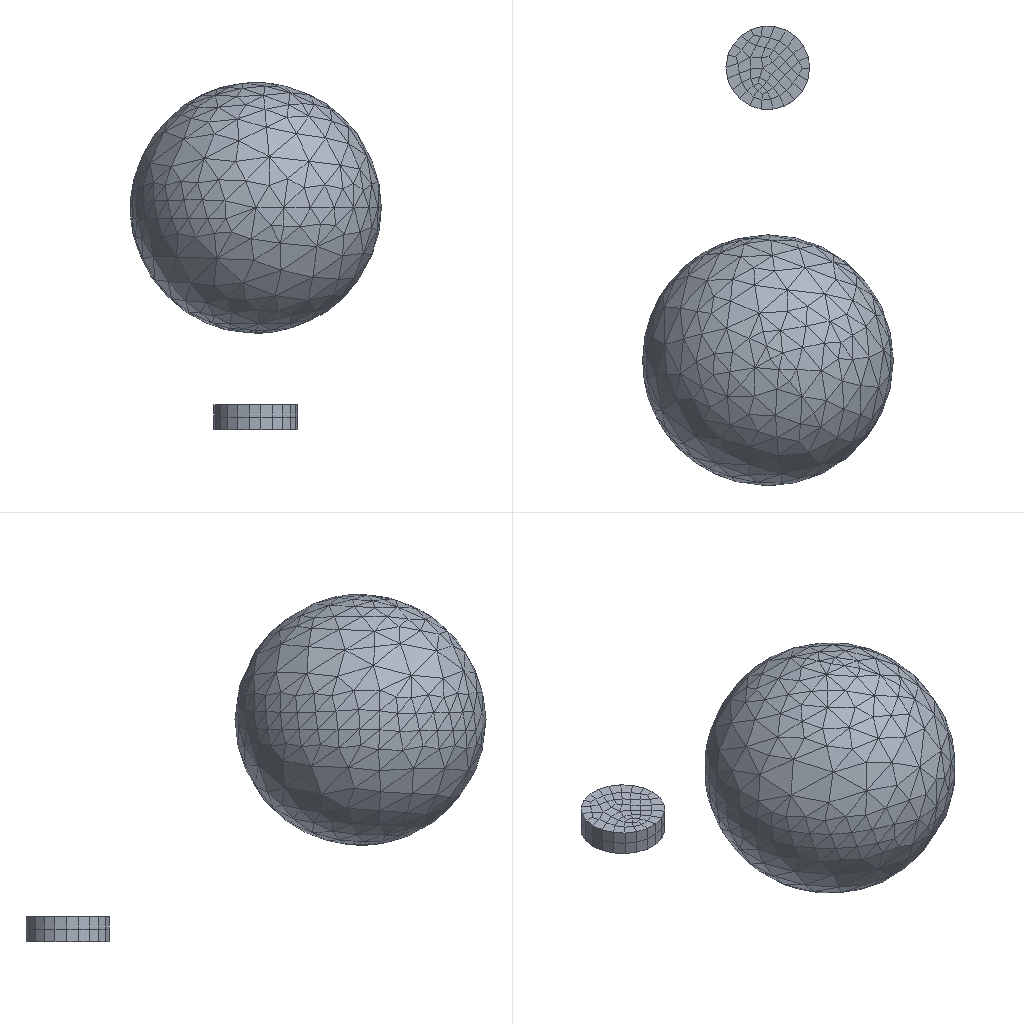Simulation study | abaqus
Set-up summary:
category,name,step,type,value,unit,region
solver,abaqus
solver,version,,,Abaqus/Explicit 2020
units,not stated in the deck,,not stated
analysis,deck,,transient,transient
load_step,Step-1,Step-1,transient
load_step,requested,,,1
mesh,nodes,,,6310
mesh,elements,,,4417
element_type,R3D4,,rigid,116
element_type,T3D2,,truss,568
element_type,C3D8R,,solid,116
element_type,C3D10M,,solid,3617
load,load commands in deck,,count,2
bc,support commands in deck,,count,7
material,RUBBER,,in results
material,STRING,,in results
check,setup vs results,,match,"per instance, exact: element labels, types and connectivity; labels of the nodes the elements use; coordinates of those nodes at SINGLE_PRECISION in 3 of 5 instance(s)"
Abaqus input file, long lists of numbers shortened:
*Heading
** Job name: Job-2 Model name: tennis_gcont
** Generated by: Abaqus/CAE 2020
*Preprint, echo=NO, model=NO, history=NO, contact=NO
**
** PARTS
**
*Part, name=FRAME
*Node
    105,  -2.16,  -7.3,           0.
    106,        -1.62,  -7.825,           0.
** (173 more lines like these left out)
*Element, type=R3D4
3001,   105,   106, 10106, 10105
3002,   106,   107, 10107, 10106
** (114 more lines like these left out)
*Nset, nset=FRAME-RefPt_, internal
 10000,
*End Part
**
*Part, name=PART-1
*Node
    104,  -2.7,       -6.625,           0.
    105,  -2.16,  -7.3,           0.
** (329 more lines like these left out)
*Element, type=T3D2
   1,  204,  205
   2,  205,  206
** (566 more lines like these left out)
*Elset, elset=STRINGS
    1,    2,    3,    4,    5,    6,    7,    8,    9,   10,   11,   12,   13,   14,   15,   16
   17,   18,   19,   20,   21,   22,   23,   24,   25,   26,   27,   28,   29,   30,   31,   32
** (34 more lines like these left out)
*Elset, elset=Set-6
    1,    2,    3,    4,    5,    6,    7,    8,    9,   10,   11,   12,   13,   14,   15,   16
   17,   18,   19,   20,   21,   22,   23,   24,   25,   26,   27,   28,   29,   30,   31,   32
** (34 more lines like these left out)
*Elset, elset=Set-7
    1,    2,    3,    4,    5,    6,    7,    8,    9,   10,   11,   12,   13,   14,   15,   16
   17,   18,   19,   20,   21,   22,   23,   24,   25,   26,   27,   28,   29,   30,   31,   32
** (34 more lines like these left out)
** Section: Section-1-STRINGS
*Solid Section, elset=Set-7, material=STRING
0.007854,
*End Part
**
*Part, name=bizhen
*Node
      1,  0.4153, -0.2784,           0.
      2,  0.4769, -0.1501,           0.
** (138 more lines like these left out)
*Element, type=C3D8R
 1,  93,  90,  89,  94,  23,  20,  19,  24
 2,  94,  89,  88,  95,  24,  19,  18,  25
** (56 more lines like these left out)
*Nset, nset=Set-2, generate
   1,  140,    1
*Elset, elset=Set-2, generate
  1,  58,   1
** Section: Section-bizhen
*Solid Section, elset=Set-2, material=RUBBER
,
*End Part
**
*Part, name=qiu
*Node
      1,  0.3338,   1.462,           0.
      2,   0.6508,    1.351,           0.
** (5522 more lines like these left out)
*Element, type=C3D10M
   1,  337,  338,  339,  340,  790,  789,  788,  792,  791,  793
   2,  337,  341,  342,  343,  796,  795,  794,  798,  797,  799
** (3615 more lines like these left out)
*Nset, nset=Set-7, generate
    1,  5524,     1
*Elset, elset=Set-7, generate
    1,  3617,     1
*Nset, nset=Set-8, generate
    1,  5524,     1
*Elset, elset=Set-8, generate
    1,  3617,     1
** Section: Section-bizhen
*Solid Section, elset=Set-8, material=RUBBER
,
*End Part
**
**
** ASSEMBLY
**
*Assembly, name=Assembly
**
*Instance, name=FRAME-1, part=FRAME
*End Instance
**
*Instance, name=PART-1-1, part=PART-1
*End Instance
**
*Instance, name=bizhen-1, part=bizhen
          0.,          3.5,           0.
*End Instance
**
*Instance, name=bizhen-1-lin-2-1, part=bizhen
          0.,          3.5,        -0.15
*End Instance
**
*Instance, name=qiu-1, part=qiu
          0.,           0.,          2.5
*End Instance
**
*Node
      1,          1.5,           0.,          2.5
*Node
      2,           0.,           0.,           0.
*Nset, nset=BACK, instance=FRAME-1
 20105, 20106, 20107, 20108, 20109, 20110, 20111, 20112, 20113, 20204, 20214, 20303, 20315, 20402, 20416, 20501
 20517, 20601, 20617, 20701, 20717, 20801, 20817, 20901, 20917, 21001, 21017, 21101, 21117, 21201, 21217, 21301
** (2 more lines like these left out)
*Elset, elset=FRAME, instance=FRAME-1
 3001, 3002, 3003, 3004, 3005, 3006, 3007, 3008, 3009, 3010, 3011, 3012, 3013, 3014, 3015, 3016
 3017, 3018, 3019, 3020, 3021, 3022, 3023, 3024, 3025, 3036, 3037, 3038, 3039, 3040, 3041, 3042
** (6 more lines like these left out)
*Nset, nset=FRONT, instance=FRAME-1
 10105, 10106, 10107, 10108, 10109, 10110, 10111, 10112, 10113, 10204, 10214, 10303, 10315, 10402, 10416, 10501
 10517, 10601, 10617, 10701, 10717, 10801, 10817, 10901, 10917, 11001, 11017, 11101, 11117, 11201, 11217, 11301
** (2 more lines like these left out)
*Nset, nset=MIDPLANE, instance=FRAME-1
  105,  106,  107,  108,  109,  110,  111,  112,  113,  204,  214,  303,  315,  402,  416,  501
  517,  601,  617,  701,  717,  801,  817,  901,  917, 1001, 1017, 1101, 1117, 1201, 1217, 1301
** (2 more lines like these left out)
*Nset, nset=MIDPLANE, instance=PART-1-1
  105,  106,  107,  108,  109,  110,  111,  112,  113,  204,  214,  303,  315,  402,  416,  501
  517,  601,  617,  701,  717,  801,  817,  901,  917, 1001, 1017, 1101, 1117, 1201, 1217, 1301
** (2 more lines like these left out)
*Nset, nset=N200, instance=PART-1-1, generate
 204,  214,    1
*Nset, nset=N200, instance=FRAME-1
 204, 214
*Nset, nset=N500, instance=PART-1-1, generate
 502,  516,    1
*Nset, nset=N1900, instance=FRAME-1
 1902, 1916
*Nset, nset=N1900, instance=PART-1-1, generate
 1902,  1916,     1
*Nset, nset=NCONTACT, instance=PART-1-1
  205,  206,  207,  208,  209,  210,  211,  212,  213,  304,  305,  306,  307,  308,  309,  310
  311,  312,  313,  314,  403,  404,  405,  406,  407,  408,  409,  410,  411,  412,  413,  414
** (15 more lines like these left out)
*Nset, nset=STRINGS, instance=PART-1-1
  205,  206,  207,  208,  209,  210,  211,  212,  213,  304,  305,  306,  307,  308,  309,  310
  311,  312,  313,  314,  403,  404,  405,  406,  407,  408,  409,  410,  411,  412,  413,  414
** (15 more lines like these left out)
*Nset, nset=Set-14, instance=PART-1-1
  104,  105,  106,  107,  108,  109,  110,  111,  112,  113,  114,  204,  214,  303,  315,  402
  416,  501,  517,  601,  617,  701,  717,  801,  817,  901,  917, 1001, 1017, 1101, 1117, 1201
** (2 more lines like these left out)
*Nset, nset=Set-16, instance=bizhen-1, generate
  71,  140,    1
*Nset, nset=Set-16, instance=bizhen-1-lin-2-1, generate
  1,  70,   1
*Elset, elset=Set-16, instance=bizhen-1, generate
  1,  58,   1
*Elset, elset=Set-16, instance=bizhen-1-lin-2-1, generate
  1,  58,   1
*Nset, nset=Set-17, instance=qiu-1
    1,    2,    3,    4,    5,    6,    7,    8,    9,   10,   11,   12,   13,   14,   15,   16
   17,   18,   19,   20,   21,   22,   23,   24,   25,   26,   27,   28,   29,   30,   31,   32
** (82 more lines like these left out)
*Elset, elset=Set-17, instance=qiu-1
   30,  101,  125,  183,  237,  261,  262,  300,  315,  360,  375,  402,  438,  457,  461,  463
  495,  523,  546,  557,  576,  578,  599,  694,  728,  756,  765,  767,  781,  797,  799,  873
** (40 more lines like these left out)
*Nset, nset=Set-21
 1,
*Nset, nset=U, instance=PART-1-1
 1209,
*Nset, nset=_Ref-Pt_FRAME-1_10000, internal, instance=FRAME-1
 10000,
*Nset, nset=b_Set-19, instance=qiu-1, generate
    1,  5524,     1
*Elset, elset=b_Set-19, instance=qiu-1, generate
    1,  3617,     1
*Nset, nset=s_Set-15, instance=PART-1-1
 1808, 1809, 1810, 1908, 1909, 1910
*Nset, nset=s_Set-18, instance=FRAME-1
 10000,
*Nset, nset=s_Set-18, instance=PART-1-1
  604,  605,  606,  607,  608,  609,  610,  611,  612,  613,  614,  704,  705,  706,  707,  708
  709,  710,  711,  712,  713,  714,  804,  805,  806,  807,  808,  809,  810,  811,  812,  813
** (6 more lines like these left out)
*Nset, nset=_M20, internal, instance=FRAME-1
 10000,
*Nset, nset=_PickedSet55, internal
 1,
*Elset, elset=_Surf-5_S1, internal, instance=bizhen-1, generate
  1,  58,   1
*Elset, elset=_Surf-5_S2, internal, instance=bizhen-1-lin-2-1, generate
  1,  58,   1
*Surface, type=ELEMENT, name=Surf-5
_Surf-5_S1, S1
_Surf-5_S2, S2
*Elset, elset=_m_Surf-2_S1, internal, instance=bizhen-1-lin-2-1, generate
  1,  58,   1
*Surface, type=ELEMENT, name=m_Surf-2
_m_Surf-2_S1, S1
*Elset, elset=_m_Surf-3_S2, internal, instance=bizhen-1, generate
  1,  58,   1
*Elset, elset=_m_Surf-3_S1, internal, instance=bizhen-1-lin-2-1, generate
  1,  58,   1
*Surface, type=ELEMENT, name=m_Surf-3
_m_Surf-3_S2, S2
_m_Surf-3_S1, S1
*Elset, elset=_m_Surf-4_S3, internal, instance=qiu-1
   30,  101,  125,  183,  237,  261,  262,  300,  315,  360,  375,  402,  438,  457,  461,  463
  495,  546,  557,  576,  578,  599,  694,  756,  765,  797,  873,  885,  925, 1128, 1129, 1145
** (36 more lines like these left out)
*Elset, elset=_m_Surf-4_S4, internal, instance=qiu-1
  523,  728,  767,  781,  799,  961, 1518, 1663, 1748, 1814, 2113, 2189, 2192, 2245, 2307, 2361
 2378, 2468, 2513, 2752, 2792, 2843, 2898, 2921, 2935, 2954, 2989, 3065, 3121, 3156, 3238, 3251
** (1 more lines like these left out)
*Elset, elset=_m_Surf-4_S2, internal, instance=qiu-1
 1138, 1678, 1707, 1821, 1857, 1941, 2072, 2100, 2139, 2158, 2196, 2605, 2639, 2663, 2720, 2723
 2748, 2807, 2879, 2924, 3164, 3393, 3426, 3476, 3603
*Elset, elset=_m_Surf-4_S1, internal, instance=qiu-1
 1455, 1842, 1976, 2384, 2805, 2823, 2945, 3295, 3415
*Surface, type=ELEMENT, name=m_Surf-4
_m_Surf-4_S3, S3
_m_Surf-4_S4, S4
_m_Surf-4_S2, S2
_m_Surf-4_S1, S1
*Elset, elset=_m_Surf-6_S1, internal, instance=bizhen-1-lin-2-1, generate
  1,  58,   1
*Surface, type=ELEMENT, name=m_Surf-6
_m_Surf-6_S1, S1
*Elset, elset=_s_Surf-6_S2, internal, instance=bizhen-1, generate
  1,  58,   1
*Surface, type=ELEMENT, name=s_Surf-6
_s_Surf-6_S2, S2
*Surface, type=NODE, name=s_Set-15_CNS_, internal
s_Set-15, 1.
** Constraint: Constraint-2
*Tie, name=Constraint-2, adjust=yes
s_Set-15_CNS_, m_Surf-3
** Constraint: Constraint-3
*Rigid Body, ref node=_PickedSet55, elset=b_Set-19, position=CENTER OF MASS
** Constraint: Constraint-4
*Tie, name=Constraint-4, adjust=yes
s_Surf-6, m_Surf-6
** Constraint: RigidBody-1
*Rigid Body, ref node=_Ref-Pt_FRAME-1_10000, elset=FRAME
*End Assembly
**
** MATERIALS
**
** ******************
**
**  Material definitions.
**
** ******************
*Material, name=RUBBER
*Density
2000.,
*Elastic
 1.2e+10, 0.37
** COMMENTS FROM *DENSITY
** ======================
**
**   Nylon type 6 general purpose.
*Material, name=STRING
*Density
1000.,
*Elastic
 5e+11, 0.35
**
** INTERACTION PROPERTIES
**
*Surface Interaction, name=SPH_STRING
*Friction
 0.1,
*Surface Behavior, pressure-overclosure=HARD
**
** BOUNDARY CONDITIONS
**
** Name: Disp-BC-1 Type: 位移/转角
*Boundary
_M20, 1, 1
_M20, 2, 2
_M20, 3, 3
_M20, 4, 4
_M20, 5, 5
_M20, 6, 6
**
** PREDEFINED FIELDS
**
** Name: IC-1   Type: Stress
*Initial Conditions, type=STRESS
PART-1-1.STRINGS, 1.273e+06, 1.273e+06, 1.273e+06,
** Name: IC-3   Type: Velocity
*Initial Conditions, type=VELOCITY
Set-21, 1, 0.
Set-21, 3, -100.
**
** INTERACTIONS
**
** Interaction: Int-2
*Contact, op=NEW
*Contact Inclusions, ALL EXTERIOR
*Contact Property Assignment
 ,  , SPH_STRING
** ----------------------------------------------------------------
**
** STEP: Step-1
**
*Step, name=Step-1, nlgeom=YES
*Dynamic, Explicit
, 0.1
*Bulk Viscosity
0.06, 1.2
**
** BOUNDARY CONDITIONS
**
** Name: BC-2 Type: 对称/反对称/完全固定
*Boundary
Set-14, ENCASTRE
**
** LOADS
**
** Name: Load-1   Type: Pressure
*Dsload
Surf-5, P, 1e+06
**
** OUTPUT REQUESTS
**
*Restart, write, number interval=30, time marks=NO
**
** FIELD OUTPUT: F-Output-2
**
*Output, field
*Node Output
A, U, V
**
** FIELD OUTPUT: F-Output-1
**
*Element Output, directions=YES
S,
**
** HISTORY OUTPUT: H-Output-1
**
*Output, history, time interval=0.0001
*Node Output, nset=U
U3,
*End Step
Results summary:
result,step,Step-1,completed,increments=11693 time=0.1/0.1
result,analysis,,,transient
result,last_loadstep,,,1
result,primary field,,,U